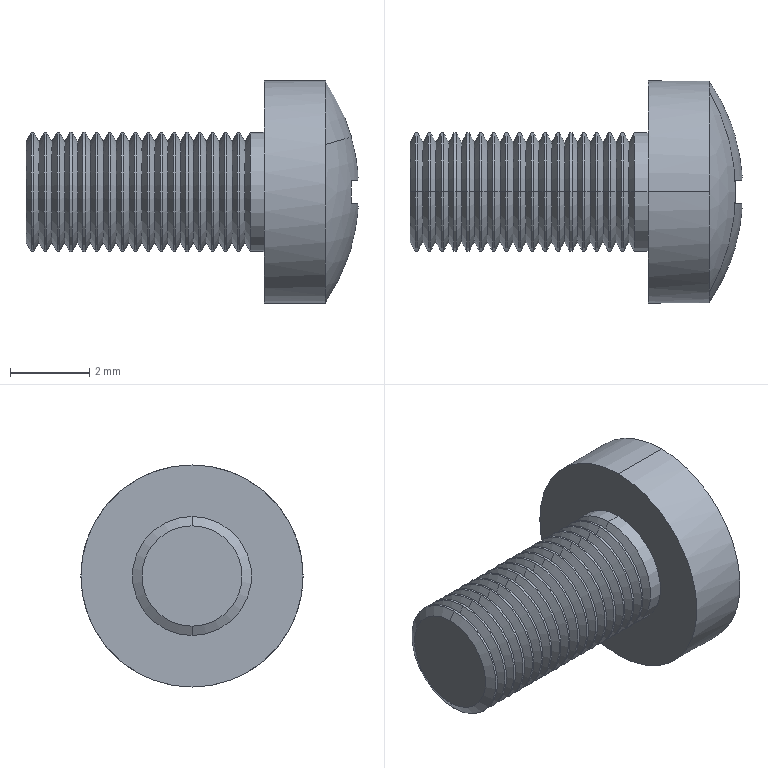Part | SolidWorks | features BaseBody 1 | 1 solid | 129 faces | box 8.37 x 5.6 x 5.6 mm | volume 82.974 mm3 | cone 70 | cylinder 42 | plane 15 | sphere 2 | commonest cylinder face diameters 3 x36 0.6 x4 5.6 x2